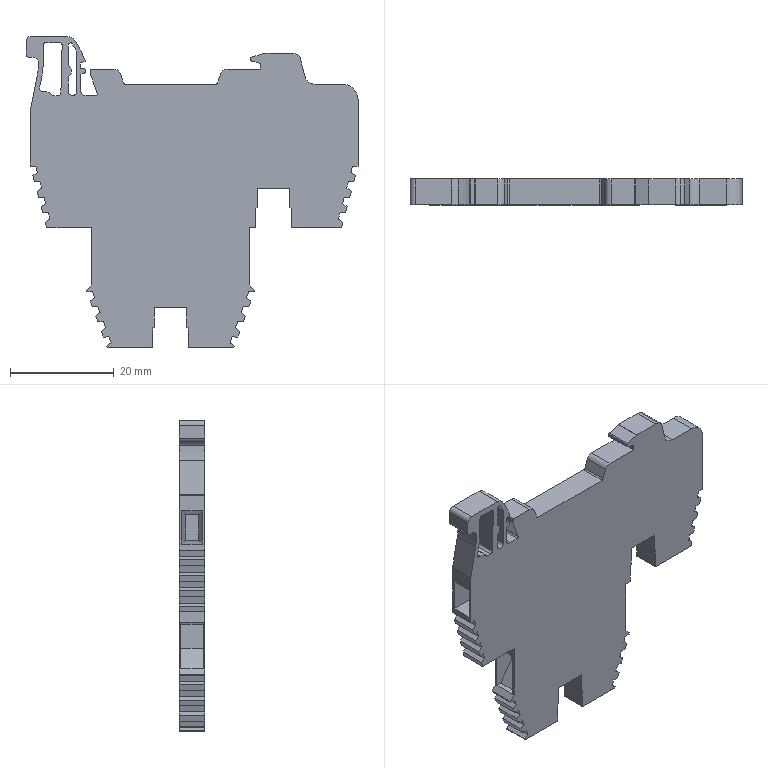Part | SolidWorks | features BaseBody 1 | 1 solid | 239 faces | box 64.028 x 5 x 60 mm | volume 11357 mm3 | plane 196 | cylinder 43 | commonest cylinder face diameters 1 x8 3.75 x7 0.6 x6 0.4 x3 2 x3 1.2 x2